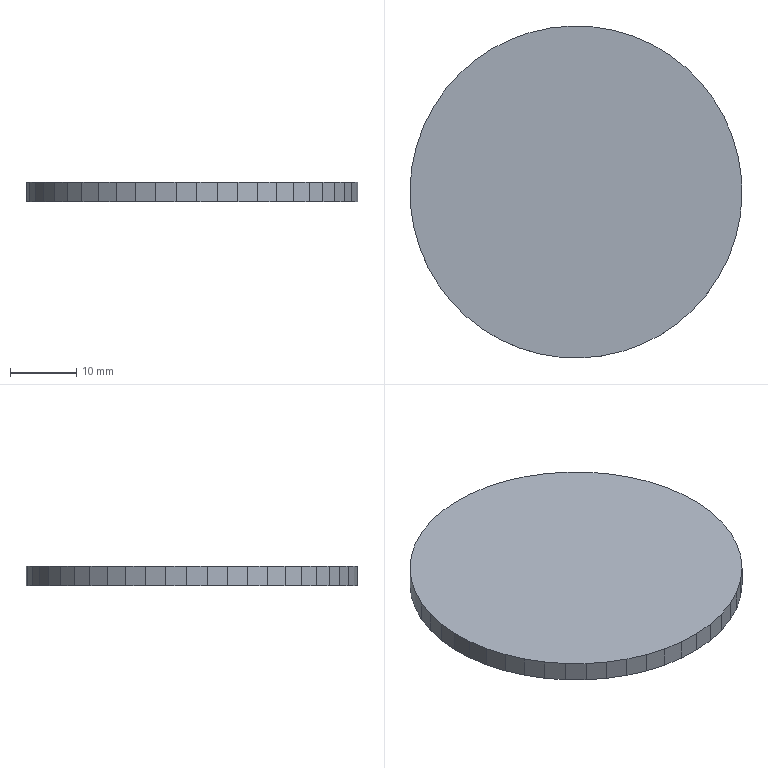Part | SolidWorks | features Extrusion 1 | 1 solid | 52 faces | box 49.972 x 49.978 x 3 mm | volume 5875 mm3 | plane 52